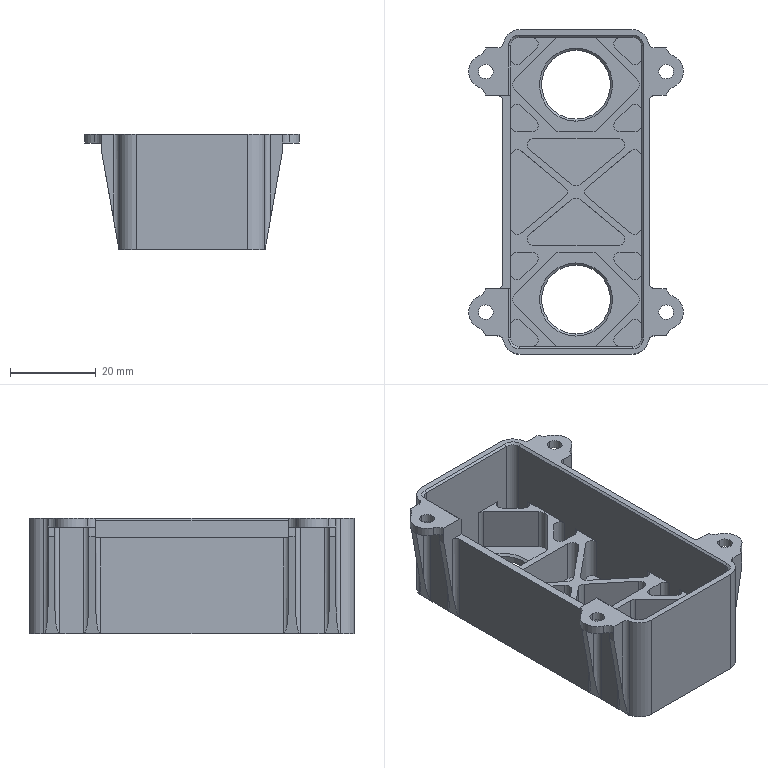NC program | NX | posted with a generic post | part box 50 x 75.58 x 26.8 mm
Whole program:
N10 G17 G21 G94 G90
(FLOOR_WALL_COPY_1_COPY , TOOL : D4)
N12 T11 M6
N14 G54
N16 G17 G0 G90 X-12.796 Y33.703 S9500 M3
N18 G43 Z30. H11
N20 Z-13.8
N22 G94 G1 Z-14.8 F1100.
N24 G41 X-12.846 Y33.79 D11
N26 X-12.894 Y33.847
N28 G3 X-13.2 Y33.99 R0.4
N30 G1 Y-33.99
N32 X13.2
N34 Y33.99
N36 X-13.2
N38 G3 X-13.057 Y33.684 R0.4
N40 G1 X-13. Y33.636
N42 G40
N44 X-12.913 Y33.586
N46 Z-13.8
N48 G0 Z30.
N50 X-12.953 Y32.863
N52 Z-23.8
N54 G1 Z-24.8
N56 G41 X-13. Y32.775
N58 X-13.057 Y32.598
N60 G3 X-13.2 Y32.292 R0.4
N62 G1 X-11.502 Y33.99
N64 X-13.2
N66 Y32.292
N68 G3 X-13.084 Y32.61 R0.4
N70 G1 X-13. Y32.775
N72 G40
N74 X-12.971 Y32.87
N76 Z-23.8
N78 G0 Z30.
N80 X-3.319 Y33.703
N82 Z-23.8
N84 G1 Z-24.8
N86 G41 X-3.369 Y33.79
N88 X-3.417 Y33.847
N90 G3 X-3.724 Y33.99 R0.4
N92 G1 X-12.714 Y25.
N94 X-3.714 Y16.
N96 X3.714
N98 X12.714 Y25.
N100 X3.724 Y33.99
N102 X-3.724
N104 G3 X-3.839 Y33.672 R0.4
N106 G1 X-3.833 Y33.598
N108 G40
N110 X-3.807 Y33.501
N112 Z-23.8
N114 G0 Z30.
N116 X12.073 Y33.743
N118 Z-23.8
N120 G1 Z-24.8
N122 G41 X11.985 Y33.79
N124 X11.808 Y33.847
N126 G3 X11.502 Y33.99 R0.4
N128 G1 X13.2 Y32.292
N130 Y33.99
N132 X11.502
N134 G3 X11.82 Y33.874 R0.4
N136 G1 X11.985 Y33.79
N138 G40
N140 X12.08 Y33.761
N142 Z-23.8
N144 G0 Z30.
N146 X-12.073 Y-33.743
N148 Z-23.8
N150 G1 Z-24.8
N152 G41 X-11.985 Y-33.79
N154 X-11.808 Y-33.847
N156 G3 X-11.502 Y-33.99 R0.4
N158 G1 X-13.2 Y-32.292
N160 Y-33.99
N162 X-11.502
N164 G3 X-11.82 Y-33.874 R0.4
N166 G1 X-11.985 Y-33.79
N168 G40
N170 X-12.08 Y-33.761
N172 Z-23.8
N174 G0 Z30.
N176 X-12.063 Y16.247
N178 Z-23.8
N180 G1 Z-24.8
N182 G41 X-11.975 Y16.2
N184 X-11.798 Y16.143
N186 G3 X-11.492 Y16. R0.4
N188 G1 X-13.2 Y17.708
N190 Y16.
N192 X-11.492
N194 G3 X-11.81 Y16.116 R0.4
N196 G1 X-11.975 Y16.2
N198 G40
N200 X-12.07 Y16.229
N202 Z-23.8
N204 G0 Z30.
N206 X7.785 Y10.271
N208 Z-23.8
N210 G1 Z-24.8
N212 G41 X7.88 Y10.3
N214 X8.111 Y10.416
N216 G3 X8.438 Y10.5 R0.4
N218 G1 X-8.438
N220 X0. Y3.56
N222 X8.438 Y10.5
N224 G3 X8.132 Y10.357 R0.4
N226 G1 X7.88 Y10.3
N228 G40
N230 X7.788 Y10.261
N232 Z-23.8
N234 G0 Z30.
N236 X-12.975 Y6.775
N238 Z-23.8
N240 G1 Z-24.8
N242 G41 X-13. Y6.871
N244 X-13.054 Y6.99
N246 G3 X-13.2 Y7.295 R0.4
N248 G1 Y-7.295
N250 X-4.33 Y0.
N252 X-13.2 Y7.295
N254 G3 X-13.057 Y6.988 R0.4
N256 G1 X-13. Y6.871
N258 G40
N260 X-12.941 Y6.79
N262 Z-23.8
N264 G0 Z30.
N266 X12.953 Y17.137
N268 Z-23.8
N270 G1 Z-24.8
N272 G41 X13. Y17.225
N274 X13.057 Y17.402
N276 G3 X13.2 Y17.708 R0.4
N278 G1 X11.492 Y16.
N280 X13.2
N282 Y17.708
N284 G3 X13.084 Y17.39 R0.4
N286 G1 X13. Y17.225
N288 G40
N290 X12.971 Y17.13
N292 Z-23.8
N294 G0 Z30.
N296 X3.319 Y-33.703
N298 Z-23.8
N300 G1 Z-24.8
N302 G41 X3.369 Y-33.79
N304 X3.417 Y-33.847
N306 G3 X3.724 Y-33.99 R0.4
N308 G1 X12.714 Y-25.
N310 X3.714 Y-16.
N312 X-3.714
N314 X-12.714 Y-25.
N316 X-3.724 Y-33.99
N318 X3.724
N320 G3 X3.839 Y-33.672 R0.4
N322 G1 X3.833 Y-33.598
N324 G40
N326 X3.807 Y-33.501
N328 Z-23.8
N330 G0 Z30.
N332 X-7.785 Y-10.271
N334 Z-23.8
N336 G1 Z-24.8
N338 G41 X-7.88 Y-10.3
N340 X-8.111 Y-10.416
N342 G3 X-8.438 Y-10.5 R0.4
N344 G1 X8.438
N346 X0. Y-3.56
N348 X-8.438 Y-10.5
N350 G3 X-8.132 Y-10.357 R0.4
N352 G1 X-7.88 Y-10.3
N354 G40
N356 X-7.788 Y-10.261
N358 Z-23.8
N360 G0 Z30.
N362 X-12.953 Y-17.137
N364 Z-23.8
N366 G1 Z-24.8
N368 G41 X-13. Y-17.225
N370 X-13.057 Y-17.402
N372 G3 X-13.2 Y-17.708 R0.4
N374 G1 X-11.492 Y-16.
N376 X-13.2
N378 Y-17.708
N380 G3 X-13.084 Y-17.39 R0.4
N382 G1 X-13. Y-17.225
N384 G40
N386 X-12.971 Y-17.13
N388 Z-23.8
N390 G0 Z30.
N392 X12.975 Y-6.775
N394 Z-23.8
N396 G1 Z-24.8
N398 G41 X13. Y-6.871
N400 X13.054 Y-6.99
N402 G3 X13.2 Y-7.295 R0.4
N404 G1 Y7.295
N406 X4.33 Y0.
N408 X13.2 Y-7.295
N410 G3 X13.057 Y-6.988 R0.4
N412 G1 X13. Y-6.871
N414 G40
N416 X12.941 Y-6.79
N418 Z-23.8
N420 G0 Z30.
N422 X12.063 Y-16.247
N424 Z-23.8
N426 G1 Z-24.8
N428 G41 X11.975 Y-16.2
N430 X11.798 Y-16.143
N432 G3 X11.492 Y-16. R0.4
N434 G1 X13.2 Y-17.708
N436 Y-16.
N438 X11.492
N440 G3 X11.81 Y-16.116 R0.4
N442 G1 X11.975 Y-16.2
N444 G40
N446 X12.07 Y-16.229
N448 Z-23.8
N450 G0 Z30.
N452 X12.953 Y-32.863
N454 Z-23.8
N456 G1 Z-24.8
N458 G41 X13. Y-32.775
N460 X13.057 Y-32.598
N462 G3 X13.2 Y-32.292 R0.4
N464 G1 X11.502 Y-33.99
N466 X13.2
N468 Y-32.292
N470 G3 X13.084 Y-32.61 R0.4
N472 G1 X13. Y-32.775
N474 G40
N476 X12.971 Y-32.87
N478 Z-23.8
N480 G0 Z30.
N482 M5
N484 M2